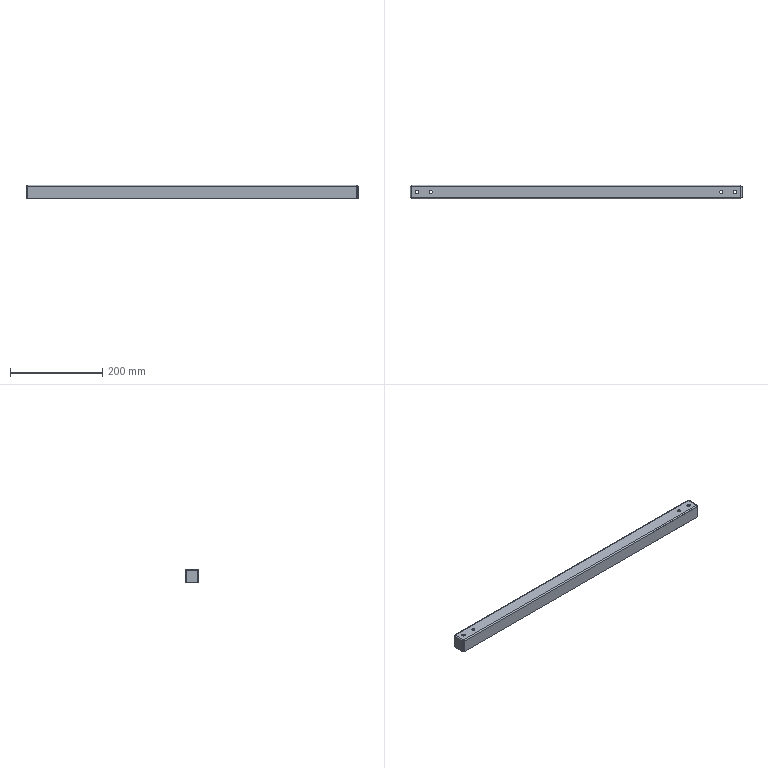Part | STEP file | Middle sheet metal support plate | 1 solid | 46 faces | box 720 x 30 x 30 mm | volume 93836 mm3 | plane 22 | cylinder 16 | spline 8 | commonest cylinder face diameters 7 x8 2 x4 5 x4